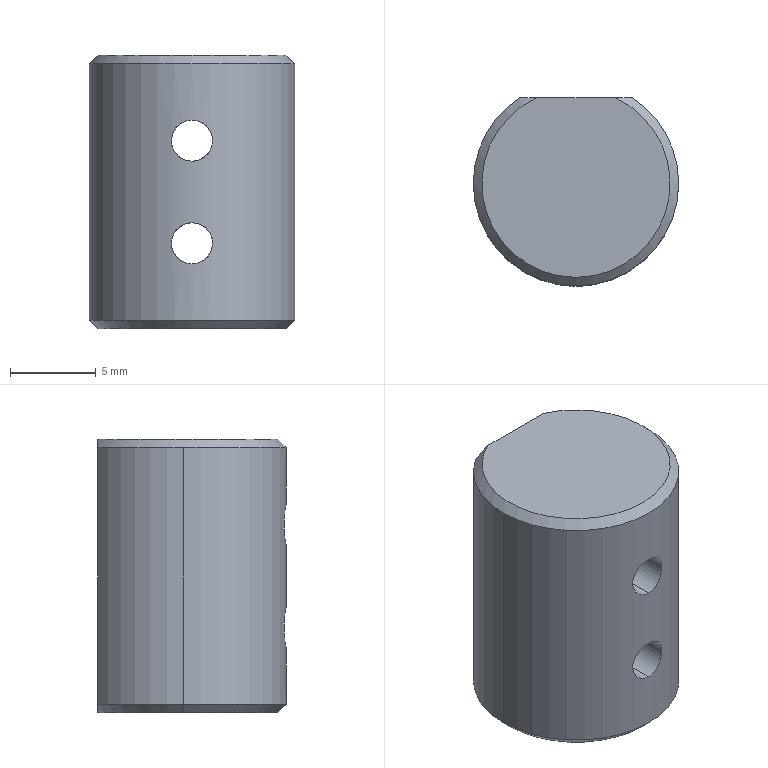Part | STEP file | Guide rod connection | 1 solid | 20 faces | box 12 x 11 x 16 mm | volume 1579 mm3 | cylinder 11 | plane 5 | cone 4 | commonest cylinder face diameters 2.4 x4 4.4 x4 12 x3